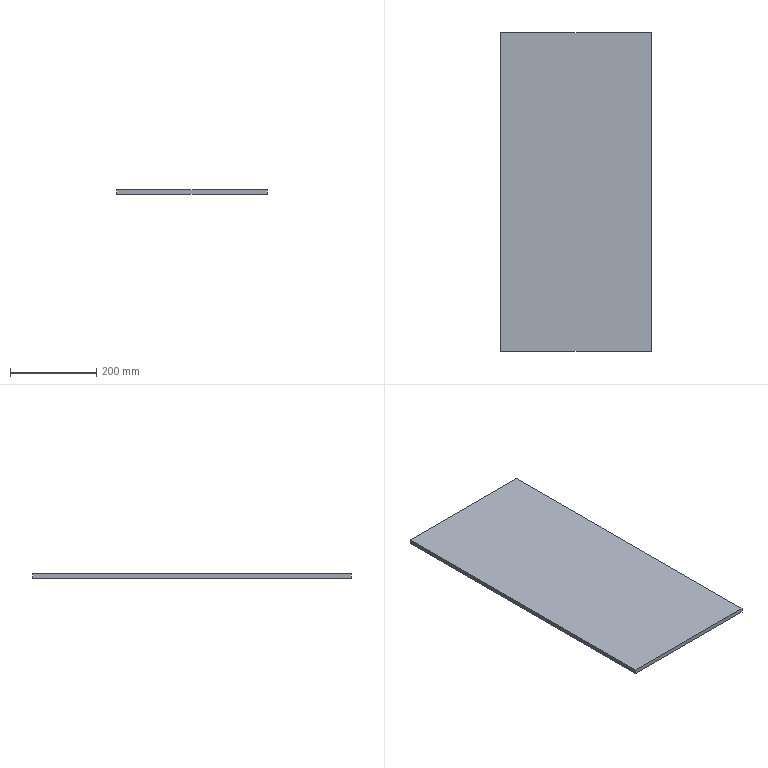Part | STEP file | 16-Steel plate | 1 solid | 6 faces | box 350 x 740 x 10 mm | volume 2590000 mm3 | plane 6
STEP:
#1=CARTESIAN_POINT('',(0.,0.,0.));
#2=DIRECTION('',(0.,0.,1.));
#3=DIRECTION('',(1.,0.,0.));
#4=AXIS2_PLACEMENT_3D('',#1,#2,#3);
#5=CARTESIAN_POINT('',(0.,0.,0.));
#6=VERTEX_POINT('',#5);
#7=CARTESIAN_POINT('',(0.,-740.,0.));
#8=VERTEX_POINT('',#7);
#9=CARTESIAN_POINT('',(0.,0.,0.));
#10=DIRECTION('',(0.,-1.,0.));
#11=VECTOR('',#10,1.);
#12=LINE('',#9,#11);
#13=CARTESIAN_POINT('',(0.,0.,10.));
#14=DIRECTION('',(1.,0.,0.));
#15=DIRECTION('',(0.,1.,0.));
#16=AXIS2_PLACEMENT_3D('',#13,#14,#15);
#17=PLANE('',#16);
#18=CARTESIAN_POINT('',(0.,-10.));
#19=DIRECTION('',(-1.,0.));
#20=VECTOR('',#19,1.);
#21=LINE('',#18,#20);
#22=(GEOMETRIC_REPRESENTATION_CONTEXT(2)PARAMETRIC_REPRESENTATION_CONTEXT()REPRESENTATION_CONTEXT('',''));
#23=DEFINITIONAL_REPRESENTATION('',(#21),#22);
#24=PCURVE('',#17,#23);
#25=CARTESIAN_POINT('',(0.,0.,0.));
#26=DIRECTION('',(0.,0.,1.));
#27=DIRECTION('',(1.,0.,0.));
#28=AXIS2_PLACEMENT_3D('',#25,#26,#27);
#29=PLANE('',#28);
#30=CARTESIAN_POINT('',(0.,0.));
#31=DIRECTION('',(0.,-1.));
#32=VECTOR('',#31,1.);
#33=LINE('',#30,#32);
#34=(GEOMETRIC_REPRESENTATION_CONTEXT(2)PARAMETRIC_REPRESENTATION_CONTEXT()REPRESENTATION_CONTEXT('',''));
#35=DEFINITIONAL_REPRESENTATION('',(#33),#34);
#36=PCURVE('',#29,#35);
#37=SURFACE_CURVE('',#12,(#24,#36),.PCURVE_S1.);
#38=EDGE_CURVE('',#6,#8,#37,.T.);
#39=ORIENTED_EDGE('',*,*,#38,.T.);
#40=CARTESIAN_POINT('',(0.,-740.,10.));
#41=VERTEX_POINT('',#40);
#42=CARTESIAN_POINT('',(0.,-740.,10.));
#43=DIRECTION('',(0.,0.,-1.));
#44=VECTOR('',#43,1.);
#45=LINE('',#42,#44);
#46=CARTESIAN_POINT('',(-740.,0.));
#47=DIRECTION('',(0.,-1.));
#48=VECTOR('',#47,1.);
#49=LINE('',#46,#48);
#50=(GEOMETRIC_REPRESENTATION_CONTEXT(2)PARAMETRIC_REPRESENTATION_CONTEXT()REPRESENTATION_CONTEXT('',''));
#51=DEFINITIONAL_REPRESENTATION('',(#49),#50);
#52=PCURVE('',#17,#51);
#53=CARTESIAN_POINT('',(0.,-740.,10.));
#54=DIRECTION('',(0.,1.,0.));
#55=DIRECTION('',(0.,0.,1.));
#56=AXIS2_PLACEMENT_3D('',#53,#54,#55);
#57=PLANE('',#56);
#58=CARTESIAN_POINT('',(0.,0.));
#59=DIRECTION('',(-1.,0.));
#60=VECTOR('',#59,1.);
#61=LINE('',#58,#60);
#62=(GEOMETRIC_REPRESENTATION_CONTEXT(2)PARAMETRIC_REPRESENTATION_CONTEXT()REPRESENTATION_CONTEXT('',''));
#63=DEFINITIONAL_REPRESENTATION('',(#61),#62);
#64=PCURVE('',#57,#63);
#65=SURFACE_CURVE('',#45,(#52,#64),.PCURVE_S1.);
#66=EDGE_CURVE('',#41,#8,#65,.T.);
#67=ORIENTED_EDGE('',*,*,#66,.F.);
#68=CARTESIAN_POINT('',(0.,0.,10.));
#69=VERTEX_POINT('',#68);
#70=CARTESIAN_POINT('',(0.,0.,10.));
#71=DIRECTION('',(0.,-1.,0.));
#72=VECTOR('',#71,1.);
#73=LINE('',#70,#72);
#74=CARTESIAN_POINT('',(0.,0.));
#75=DIRECTION('',(-1.,0.));
#76=VECTOR('',#75,1.);
#77=LINE('',#74,#76);
#78=(GEOMETRIC_REPRESENTATION_CONTEXT(2)PARAMETRIC_REPRESENTATION_CONTEXT()REPRESENTATION_CONTEXT('',''));
#79=DEFINITIONAL_REPRESENTATION('',(#77),#78);
#80=PCURVE('',#17,#79);
#81=CARTESIAN_POINT('',(0.,0.,10.));
#82=DIRECTION('',(0.,0.,1.));
#83=DIRECTION('',(1.,0.,0.));
#84=AXIS2_PLACEMENT_3D('',#81,#82,#83);
#85=PLANE('',#84);
#86=CARTESIAN_POINT('',(0.,0.));
#87=DIRECTION('',(0.,-1.));
#88=VECTOR('',#87,1.);
#89=LINE('',#86,#88);
#90=(GEOMETRIC_REPRESENTATION_CONTEXT(2)PARAMETRIC_REPRESENTATION_CONTEXT()REPRESENTATION_CONTEXT('',''));
#91=DEFINITIONAL_REPRESENTATION('',(#89),#90);
#92=PCURVE('',#85,#91);
#93=SURFACE_CURVE('',#73,(#80,#92),.PCURVE_S1.);
#94=EDGE_CURVE('',#69,#41,#93,.T.);
#95=ORIENTED_EDGE('',*,*,#94,.F.);
#96=CARTESIAN_POINT('',(0.,0.,10.));
#97=DIRECTION('',(0.,0.,-1.));
#98=VECTOR('',#97,1.);
#99=LINE('',#96,#98);
#100=CARTESIAN_POINT('',(0.,0.));
#101=DIRECTION('',(0.,-1.));
#102=VECTOR('',#101,1.);
#103=LINE('',#100,#102);
#104=(GEOMETRIC_REPRESENTATION_CONTEXT(2)PARAMETRIC_REPRESENTATION_CONTEXT()REPRESENTATION_CONTEXT('',''));
#105=DEFINITIONAL_REPRESENTATION('',(#103),#104);
#106=PCURVE('',#17,#105);
#107=CARTESIAN_POINT('',(0.,0.,10.));
#108=DIRECTION('',(0.,-1.,0.));
#109=DIRECTION('',(0.,0.,-1.));
#110=AXIS2_PLACEMENT_3D('',#107,#108,#109);
#111=PLANE('',#110);
#112=CARTESIAN_POINT('',(0.,0.));
#113=DIRECTION('',(1.,0.));
#114=VECTOR('',#113,1.);
#115=LINE('',#112,#114);
#116=(GEOMETRIC_REPRESENTATION_CONTEXT(2)PARAMETRIC_REPRESENTATION_CONTEXT()REPRESENTATION_CONTEXT('',''));
#117=DEFINITIONAL_REPRESENTATION('',(#115),#116);
#118=PCURVE('',#111,#117);
#119=SURFACE_CURVE('',#99,(#106,#118),.PCURVE_S1.);
#120=EDGE_CURVE('',#69,#6,#119,.T.);
#121=ORIENTED_EDGE('',*,*,#120,.T.);
#122=EDGE_LOOP('',(#39,#67,#95,#121));
#123=FACE_BOUND('',#122,.T.);
#124=ADVANCED_FACE('',(#123),#17,.F.);
#125=CARTESIAN_POINT('',(350.,-740.,0.));
#126=VERTEX_POINT('',#125);
#127=CARTESIAN_POINT('',(0.,-740.,0.));
#128=DIRECTION('',(1.,0.,0.));
#129=VECTOR('',#128,1.);
#130=LINE('',#127,#129);
#131=CARTESIAN_POINT('',(-10.,0.));
#132=DIRECTION('',(0.,1.));
#133=VECTOR('',#132,1.);
#134=LINE('',#131,#133);
#135=(GEOMETRIC_REPRESENTATION_CONTEXT(2)PARAMETRIC_REPRESENTATION_CONTEXT()REPRESENTATION_CONTEXT('',''));
#136=DEFINITIONAL_REPRESENTATION('',(#134),#135);
#137=PCURVE('',#57,#136);
#138=CARTESIAN_POINT('',(0.,-740.));
#139=DIRECTION('',(1.,0.));
#140=VECTOR('',#139,1.);
#141=LINE('',#138,#140);
#142=(GEOMETRIC_REPRESENTATION_CONTEXT(2)PARAMETRIC_REPRESENTATION_CONTEXT()REPRESENTATION_CONTEXT('',''));
#143=DEFINITIONAL_REPRESENTATION('',(#141),#142);
#144=PCURVE('',#29,#143);
#145=SURFACE_CURVE('',#130,(#137,#144),.PCURVE_S1.);
#146=EDGE_CURVE('',#8,#126,#145,.T.);
#147=ORIENTED_EDGE('',*,*,#146,.T.);
#148=CARTESIAN_POINT('',(350.,-740.,10.));
#149=VERTEX_POINT('',#148);
#150=CARTESIAN_POINT('',(350.,-740.,10.));
#151=DIRECTION('',(0.,0.,-1.));
#152=VECTOR('',#151,1.);
#153=LINE('',#150,#152);
#154=CARTESIAN_POINT('',(0.,350.));
#155=DIRECTION('',(-1.,0.));
#156=VECTOR('',#155,1.);
#157=LINE('',#154,#156);
#158=(GEOMETRIC_REPRESENTATION_CONTEXT(2)PARAMETRIC_REPRESENTATION_CONTEXT()REPRESENTATION_CONTEXT('',''));
#159=DEFINITIONAL_REPRESENTATION('',(#157),#158);
#160=PCURVE('',#57,#159);
#161=CARTESIAN_POINT('',(350.,0.,10.));
#162=DIRECTION('',(-1.,0.,0.));
#163=DIRECTION('',(0.,-1.,0.));
#164=AXIS2_PLACEMENT_3D('',#161,#162,#163);
#165=PLANE('',#164);
#166=CARTESIAN_POINT('',(740.,0.));
#167=DIRECTION('',(0.,-1.));
#168=VECTOR('',#167,1.);
#169=LINE('',#166,#168);
#170=(GEOMETRIC_REPRESENTATION_CONTEXT(2)PARAMETRIC_REPRESENTATION_CONTEXT()REPRESENTATION_CONTEXT('',''));
#171=DEFINITIONAL_REPRESENTATION('',(#169),#170);
#172=PCURVE('',#165,#171);
#173=SURFACE_CURVE('',#153,(#160,#172),.PCURVE_S1.);
#174=EDGE_CURVE('',#149,#126,#173,.T.);
#175=ORIENTED_EDGE('',*,*,#174,.F.);
#176=CARTESIAN_POINT('',(0.,-740.,10.));
#177=DIRECTION('',(1.,0.,0.));
#178=VECTOR('',#177,1.);
#179=LINE('',#176,#178);
#180=CARTESIAN_POINT('',(0.,0.));
#181=DIRECTION('',(0.,1.));
#182=VECTOR('',#181,1.);
#183=LINE('',#180,#182);
#184=(GEOMETRIC_REPRESENTATION_CONTEXT(2)PARAMETRIC_REPRESENTATION_CONTEXT()REPRESENTATION_CONTEXT('',''));
#185=DEFINITIONAL_REPRESENTATION('',(#183),#184);
#186=PCURVE('',#57,#185);
#187=CARTESIAN_POINT('',(0.,-740.));
#188=DIRECTION('',(1.,0.));
#189=VECTOR('',#188,1.);
#190=LINE('',#187,#189);
#191=(GEOMETRIC_REPRESENTATION_CONTEXT(2)PARAMETRIC_REPRESENTATION_CONTEXT()REPRESENTATION_CONTEXT('',''));
#192=DEFINITIONAL_REPRESENTATION('',(#190),#191);
#193=PCURVE('',#85,#192);
#194=SURFACE_CURVE('',#179,(#186,#193),.PCURVE_S1.);
#195=EDGE_CURVE('',#41,#149,#194,.T.);
#196=ORIENTED_EDGE('',*,*,#195,.F.);
#197=ORIENTED_EDGE('',*,*,#66,.T.);
#198=EDGE_LOOP('',(#147,#175,#196,#197));
#199=FACE_BOUND('',#198,.T.);
#200=ADVANCED_FACE('',(#199),#57,.F.);
#201=CARTESIAN_POINT('',(350.,0.,0.));
#202=VERTEX_POINT('',#201);
#203=CARTESIAN_POINT('',(350.,0.,0.));
#204=DIRECTION('',(0.,1.,0.));
#205=VECTOR('',#204,1.);
#206=LINE('',#203,#205);
#207=CARTESIAN_POINT('',(0.,-10.));
#208=DIRECTION('',(-1.,0.));
#209=VECTOR('',#208,1.);
#210=LINE('',#207,#209);
#211=(GEOMETRIC_REPRESENTATION_CONTEXT(2)PARAMETRIC_REPRESENTATION_CONTEXT()REPRESENTATION_CONTEXT('',''));
#212=DEFINITIONAL_REPRESENTATION('',(#210),#211);
#213=PCURVE('',#165,#212);
#214=CARTESIAN_POINT('',(350.,0.));
#215=DIRECTION('',(0.,1.));
#216=VECTOR('',#215,1.);
#217=LINE('',#214,#216);
#218=(GEOMETRIC_REPRESENTATION_CONTEXT(2)PARAMETRIC_REPRESENTATION_CONTEXT()REPRESENTATION_CONTEXT('',''));
#219=DEFINITIONAL_REPRESENTATION('',(#217),#218);
#220=PCURVE('',#29,#219);
#221=SURFACE_CURVE('',#206,(#213,#220),.PCURVE_S1.);
#222=EDGE_CURVE('',#126,#202,#221,.T.);
#223=ORIENTED_EDGE('',*,*,#222,.T.);
#224=CARTESIAN_POINT('',(350.,0.,10.));
#225=VERTEX_POINT('',#224);
#226=CARTESIAN_POINT('',(350.,0.,10.));
#227=DIRECTION('',(0.,0.,-1.));
#228=VECTOR('',#227,1.);
#229=LINE('',#226,#228);
#230=CARTESIAN_POINT('',(0.,0.));
#231=DIRECTION('',(0.,-1.));
#232=VECTOR('',#231,1.);
#233=LINE('',#230,#232);
#234=(GEOMETRIC_REPRESENTATION_CONTEXT(2)PARAMETRIC_REPRESENTATION_CONTEXT()REPRESENTATION_CONTEXT('',''));
#235=DEFINITIONAL_REPRESENTATION('',(#233),#234);
#236=PCURVE('',#165,#235);
#237=CARTESIAN_POINT('',(0.,350.));
#238=DIRECTION('',(1.,0.));
#239=VECTOR('',#238,1.);
#240=LINE('',#237,#239);
#241=(GEOMETRIC_REPRESENTATION_CONTEXT(2)PARAMETRIC_REPRESENTATION_CONTEXT()REPRESENTATION_CONTEXT('',''));
#242=DEFINITIONAL_REPRESENTATION('',(#240),#241);
#243=PCURVE('',#111,#242);
#244=SURFACE_CURVE('',#229,(#236,#243),.PCURVE_S1.);
#245=EDGE_CURVE('',#225,#202,#244,.T.);
#246=ORIENTED_EDGE('',*,*,#245,.F.);
#247=CARTESIAN_POINT('',(350.,0.,10.));
#248=DIRECTION('',(0.,1.,0.));
#249=VECTOR('',#248,1.);
#250=LINE('',#247,#249);
#251=CARTESIAN_POINT('',(0.,0.));
#252=DIRECTION('',(-1.,0.));
#253=VECTOR('',#252,1.);
#254=LINE('',#251,#253);
#255=(GEOMETRIC_REPRESENTATION_CONTEXT(2)PARAMETRIC_REPRESENTATION_CONTEXT()REPRESENTATION_CONTEXT('',''));
#256=DEFINITIONAL_REPRESENTATION('',(#254),#255);
#257=PCURVE('',#165,#256);
#258=CARTESIAN_POINT('',(350.,0.));
#259=DIRECTION('',(0.,1.));
#260=VECTOR('',#259,1.);
#261=LINE('',#258,#260);
#262=(GEOMETRIC_REPRESENTATION_CONTEXT(2)PARAMETRIC_REPRESENTATION_CONTEXT()REPRESENTATION_CONTEXT('',''));
#263=DEFINITIONAL_REPRESENTATION('',(#261),#262);
#264=PCURVE('',#85,#263);
#265=SURFACE_CURVE('',#250,(#257,#264),.PCURVE_S1.);
#266=EDGE_CURVE('',#149,#225,#265,.T.);
#267=ORIENTED_EDGE('',*,*,#266,.F.);
#268=ORIENTED_EDGE('',*,*,#174,.T.);
#269=EDGE_LOOP('',(#223,#246,#267,#268));
#270=FACE_BOUND('',#269,.T.);
#271=ADVANCED_FACE('',(#270),#165,.F.);
#272=CARTESIAN_POINT('',(0.,0.,0.));
#273=DIRECTION('',(-1.,0.,0.));
#274=VECTOR('',#273,1.);
#275=LINE('',#272,#274);
#276=CARTESIAN_POINT('',(10.,0.));
#277=DIRECTION('',(0.,-1.));
#278=VECTOR('',#277,1.);
#279=LINE('',#276,#278);
#280=(GEOMETRIC_REPRESENTATION_CONTEXT(2)PARAMETRIC_REPRESENTATION_CONTEXT()REPRESENTATION_CONTEXT('',''));
#281=DEFINITIONAL_REPRESENTATION('',(#279),#280);
#282=PCURVE('',#111,#281);
#283=CARTESIAN_POINT('',(0.,0.));
#284=DIRECTION('',(-1.,0.));
#285=VECTOR('',#284,1.);
#286=LINE('',#283,#285);
#287=(GEOMETRIC_REPRESENTATION_CONTEXT(2)PARAMETRIC_REPRESENTATION_CONTEXT()REPRESENTATION_CONTEXT('',''));
#288=DEFINITIONAL_REPRESENTATION('',(#286),#287);
#289=PCURVE('',#29,#288);
#290=SURFACE_CURVE('',#275,(#282,#289),.PCURVE_S1.);
#291=EDGE_CURVE('',#202,#6,#290,.T.);
#292=ORIENTED_EDGE('',*,*,#291,.T.);
#293=ORIENTED_EDGE('',*,*,#120,.F.);
#294=CARTESIAN_POINT('',(0.,0.,10.));
#295=DIRECTION('',(-1.,0.,0.));
#296=VECTOR('',#295,1.);
#297=LINE('',#294,#296);
#298=CARTESIAN_POINT('',(0.,0.));
#299=DIRECTION('',(0.,-1.));
#300=VECTOR('',#299,1.);
#301=LINE('',#298,#300);
#302=(GEOMETRIC_REPRESENTATION_CONTEXT(2)PARAMETRIC_REPRESENTATION_CONTEXT()REPRESENTATION_CONTEXT('',''));
#303=DEFINITIONAL_REPRESENTATION('',(#301),#302);
#304=PCURVE('',#111,#303);
#305=CARTESIAN_POINT('',(0.,0.));
#306=DIRECTION('',(-1.,0.));
#307=VECTOR('',#306,1.);
#308=LINE('',#305,#307);
#309=(GEOMETRIC_REPRESENTATION_CONTEXT(2)PARAMETRIC_REPRESENTATION_CONTEXT()REPRESENTATION_CONTEXT('',''));
#310=DEFINITIONAL_REPRESENTATION('',(#308),#309);
#311=PCURVE('',#85,#310);
#312=SURFACE_CURVE('',#297,(#304,#311),.PCURVE_S1.);
#313=EDGE_CURVE('',#225,#69,#312,.T.);
#314=ORIENTED_EDGE('',*,*,#313,.F.);
#315=ORIENTED_EDGE('',*,*,#245,.T.);
#316=EDGE_LOOP('',(#292,#293,#314,#315));
#317=FACE_BOUND('',#316,.T.);
#318=ADVANCED_FACE('',(#317),#111,.F.);
#319=ORIENTED_EDGE('',*,*,#94,.T.);
#320=ORIENTED_EDGE('',*,*,#195,.T.);
#321=ORIENTED_EDGE('',*,*,#266,.T.);
#322=ORIENTED_EDGE('',*,*,#313,.T.);
#323=EDGE_LOOP('',(#319,#320,#321,#322));
#324=FACE_BOUND('',#323,.T.);
#325=ADVANCED_FACE('',(#324),#85,.T.);
#326=ORIENTED_EDGE('',*,*,#38,.F.);
#327=ORIENTED_EDGE('',*,*,#291,.F.);
#328=ORIENTED_EDGE('',*,*,#222,.F.);
#329=ORIENTED_EDGE('',*,*,#146,.F.);
#330=EDGE_LOOP('',(#326,#327,#328,#329));
#331=FACE_BOUND('',#330,.T.);
#332=ADVANCED_FACE('',(#331),#29,.F.);
#333=CLOSED_SHELL('',(#124,#200,#271,#318,#325,#332));
#334=MANIFOLD_SOLID_BREP('',#333);
#335=(LENGTH_UNIT()NAMED_UNIT(*)SI_UNIT(.MILLI.,.METRE.));
#336=UNCERTAINTY_MEASURE_WITH_UNIT(LENGTH_MEASURE(0.0000001),#335,'','');
#337=(NAMED_UNIT(*)PLANE_ANGLE_UNIT()SI_UNIT($,.RADIAN.));
#338=(NAMED_UNIT(*)SI_UNIT($,.STERADIAN.)SOLID_ANGLE_UNIT());
#339=(GEOMETRIC_REPRESENTATION_CONTEXT(3)GLOBAL_UNCERTAINTY_ASSIGNED_CONTEXT((#336))GLOBAL_UNIT_ASSIGNED_CONTEXT((#335,#337,#338))REPRESENTATION_CONTEXT('',''));
#340=ADVANCED_BREP_SHAPE_REPRESENTATION('',(#4,#334),#339);